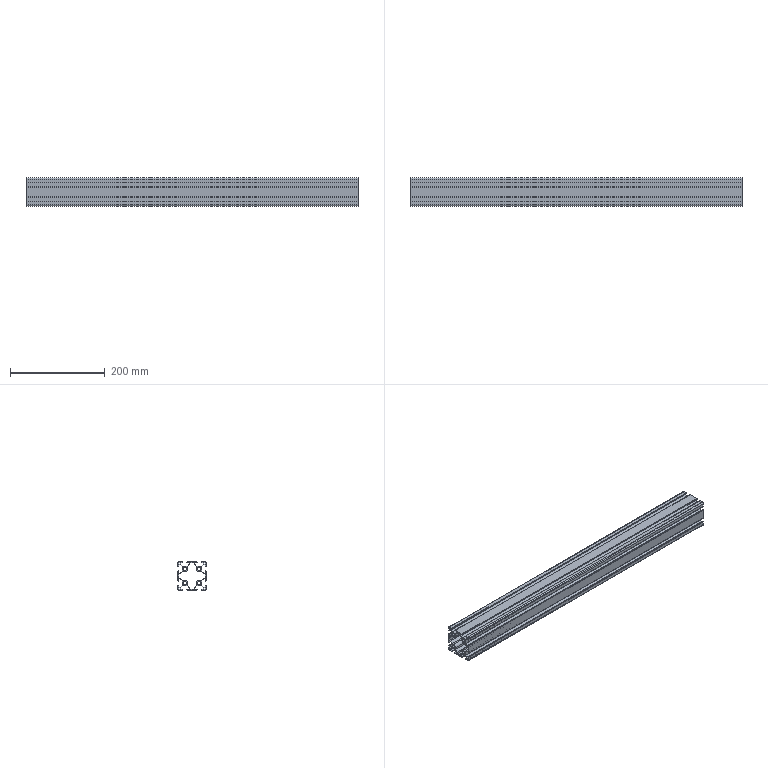Part | STEP file | PN_0007 Square aluminium tube_Default <Machined> | 1 solid | 178 faces | box 700 x 60 x 60 mm | volume 644273 mm3 | plane 162 | cylinder 16 | commonest cylinder face diameters 6.8 x8 6.76 x4 11.828 x4